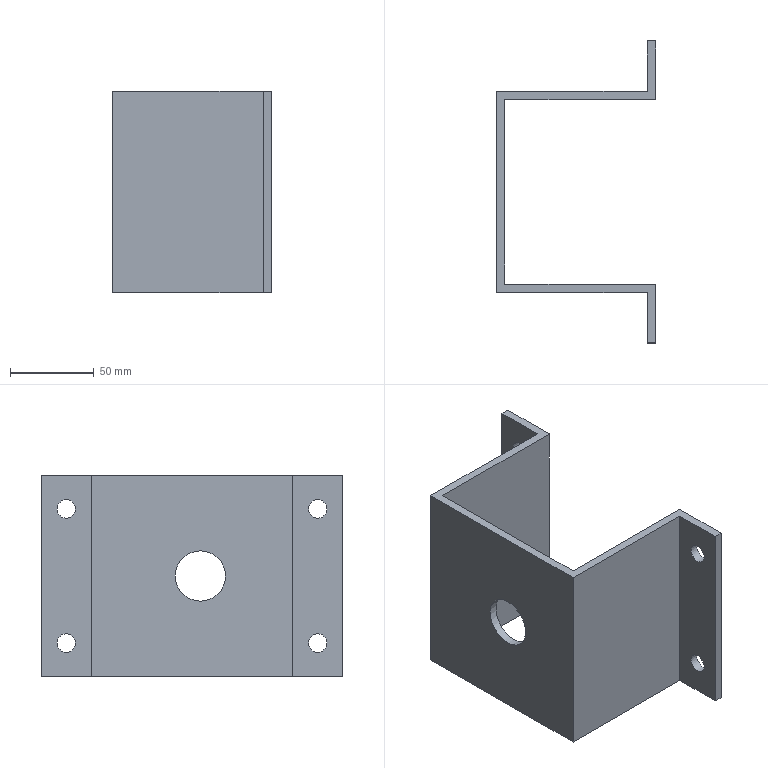Part | NX | features solid 2 | 1 solid | 19 faces | box 95 x 180 x 120 mm | volume 210565 mm3 | plane 14 | cylinder 5 | commonest cylinder face diameters 11 x4 30 x1
STEP:
#1=CARTESIAN_POINT('',(1255.,-598.,-435.));
#2=VERTEX_POINT('',#1);
#3=CARTESIAN_POINT('',(1255.,-598.,-315.));
#4=VERTEX_POINT('',#3);
#5=CARTESIAN_POINT('',(1255.,-598.,-435.));
#6=DIRECTION('',(0.,0.,1.));
#7=VECTOR('',#6,1000.);
#8=LINE('',#5,#7);
#9=EDGE_CURVE('',#2,#4,#8,.T.);
#10=ORIENTED_EDGE('',*,*,#9,.T.);
#11=CARTESIAN_POINT('',(1165.,-598.,-315.));
#12=VERTEX_POINT('',#11);
#13=CARTESIAN_POINT('',(1255.,-598.,-315.));
#14=DIRECTION('',(-1.,0.,0.));
#15=VECTOR('',#14,1000.);
#16=LINE('',#13,#15);
#17=EDGE_CURVE('',#4,#12,#16,.T.);
#18=ORIENTED_EDGE('',*,*,#17,.T.);
#19=CARTESIAN_POINT('',(1165.,-598.,-435.));
#20=VERTEX_POINT('',#19);
#21=CARTESIAN_POINT('',(1165.,-598.,-435.));
#22=DIRECTION('',(0.,0.,1.));
#23=VECTOR('',#22,1000.);
#24=LINE('',#21,#23);
#25=EDGE_CURVE('',#20,#12,#24,.T.);
#26=ORIENTED_EDGE('',*,*,#25,.F.);
#27=CARTESIAN_POINT('',(1255.,-598.,-435.));
#28=DIRECTION('',(-1.,0.,0.));
#29=VECTOR('',#28,1000.);
#30=LINE('',#27,#29);
#31=EDGE_CURVE('',#2,#20,#30,.T.);
#32=ORIENTED_EDGE('',*,*,#31,.F.);
#33=EDGE_LOOP('',(#10,#18,#26,#32));
#34=FACE_BOUND('',#33,.T.);
#35=CARTESIAN_POINT('',(1255.,-598.,-435.));
#36=DIRECTION('',(0.,1.,0.));
#37=DIRECTION('',(0.,0.,1.));
#38=AXIS2_PLACEMENT_3D('',#35,#36,#37);
#39=PLANE('',#38);
#40=ADVANCED_FACE('',(#34),#39,.F.);
#41=CARTESIAN_POINT('',(1165.,-478.,-435.));
#42=VERTEX_POINT('',#41);
#43=CARTESIAN_POINT('',(1165.,-598.,-435.));
#44=DIRECTION('',(0.,1.,0.));
#45=VECTOR('',#44,1000.);
#46=LINE('',#43,#45);
#47=EDGE_CURVE('',#20,#42,#46,.T.);
#48=ORIENTED_EDGE('',*,*,#47,.T.);
#49=CARTESIAN_POINT('',(1255.,-478.,-435.));
#50=VERTEX_POINT('',#49);
#51=CARTESIAN_POINT('',(1255.,-478.,-435.));
#52=DIRECTION('',(-1.,0.,0.));
#53=VECTOR('',#52,1000.);
#54=LINE('',#51,#53);
#55=EDGE_CURVE('',#50,#42,#54,.T.);
#56=ORIENTED_EDGE('',*,*,#55,.F.);
#57=CARTESIAN_POINT('',(1255.,-448.,-435.));
#58=VERTEX_POINT('',#57);
#59=CARTESIAN_POINT('',(1255.,-478.,-435.));
#60=DIRECTION('',(0.,-1.,0.));
#61=VECTOR('',#60,1000.);
#62=LINE('',#59,#61);
#63=EDGE_CURVE('',#50,#58,#62,.F.);
#64=ORIENTED_EDGE('',*,*,#63,.T.);
#65=CARTESIAN_POINT('',(1260.,-448.,-435.));
#66=VERTEX_POINT('',#65);
#67=CARTESIAN_POINT('',(1255.,-448.,-435.));
#68=DIRECTION('',(-1.,0.,0.));
#69=VECTOR('',#68,1000.);
#70=LINE('',#67,#69);
#71=EDGE_CURVE('',#66,#58,#70,.T.);
#72=ORIENTED_EDGE('',*,*,#71,.F.);
#73=CARTESIAN_POINT('',(1260.,-483.,-435.));
#74=VERTEX_POINT('',#73);
#75=CARTESIAN_POINT('',(1260.,-478.,-435.));
#76=DIRECTION('',(0.,-1.,0.));
#77=VECTOR('',#76,1000.);
#78=LINE('',#75,#77);
#79=EDGE_CURVE('',#66,#74,#78,.T.);
#80=ORIENTED_EDGE('',*,*,#79,.T.);
#81=CARTESIAN_POINT('',(1170.,-483.,-435.));
#82=VERTEX_POINT('',#81);
#83=CARTESIAN_POINT('',(1255.,-483.,-435.));
#84=DIRECTION('',(-1.,0.,0.));
#85=VECTOR('',#84,1000.);
#86=LINE('',#83,#85);
#87=EDGE_CURVE('',#74,#82,#86,.T.);
#88=ORIENTED_EDGE('',*,*,#87,.T.);
#89=CARTESIAN_POINT('',(1170.,-593.,-435.));
#90=VERTEX_POINT('',#89);
#91=CARTESIAN_POINT('',(1170.,-598.,-435.));
#92=DIRECTION('',(0.,1.,0.));
#93=VECTOR('',#92,1000.);
#94=LINE('',#91,#93);
#95=EDGE_CURVE('',#90,#82,#94,.T.);
#96=ORIENTED_EDGE('',*,*,#95,.F.);
#97=CARTESIAN_POINT('',(1260.,-593.,-435.));
#98=VERTEX_POINT('',#97);
#99=CARTESIAN_POINT('',(1255.,-593.,-435.));
#100=DIRECTION('',(-1.,0.,0.));
#101=VECTOR('',#100,1000.);
#102=LINE('',#99,#101);
#103=EDGE_CURVE('',#98,#90,#102,.T.);
#104=ORIENTED_EDGE('',*,*,#103,.F.);
#105=CARTESIAN_POINT('',(1260.,-628.,-435.));
#106=VERTEX_POINT('',#105);
#107=CARTESIAN_POINT('',(1260.,-598.,-435.));
#108=DIRECTION('',(0.,1.,0.));
#109=VECTOR('',#108,1000.);
#110=LINE('',#107,#109);
#111=EDGE_CURVE('',#106,#98,#110,.T.);
#112=ORIENTED_EDGE('',*,*,#111,.F.);
#113=CARTESIAN_POINT('',(1255.,-628.,-435.));
#114=VERTEX_POINT('',#113);
#115=CARTESIAN_POINT('',(1255.,-628.,-435.));
#116=DIRECTION('',(-1.,0.,0.));
#117=VECTOR('',#116,1000.);
#118=LINE('',#115,#117);
#119=EDGE_CURVE('',#106,#114,#118,.T.);
#120=ORIENTED_EDGE('',*,*,#119,.T.);
#121=CARTESIAN_POINT('',(1255.,-598.,-435.));
#122=DIRECTION('',(0.,1.,0.));
#123=VECTOR('',#122,1000.);
#124=LINE('',#121,#123);
#125=EDGE_CURVE('',#2,#114,#124,.F.);
#126=ORIENTED_EDGE('',*,*,#125,.F.);
#127=ORIENTED_EDGE('',*,*,#31,.T.);
#128=EDGE_LOOP('',(#48,#56,#64,#72,#80,#88,#96,#104,#112,#120,#126,#127));
#129=FACE_BOUND('',#128,.T.);
#130=CARTESIAN_POINT('',(1255.,-598.,-435.));
#131=DIRECTION('',(0.,0.,1.));
#132=DIRECTION('',(1.,0.,0.));
#133=AXIS2_PLACEMENT_3D('',#130,#131,#132);
#134=PLANE('',#133);
#135=ADVANCED_FACE('',(#129),#134,.F.);
#136=CARTESIAN_POINT('',(1260.,-613.,-420.5));
#137=VERTEX_POINT('',#136);
#138=CARTESIAN_POINT('',(1260.,-613.,-415.));
#139=DIRECTION('',(1.,0.,0.));
#140=DIRECTION('',(0.,0.,-1.));
#141=AXIS2_PLACEMENT_3D('',#138,#139,#140);
#142=CIRCLE('',#141,5.5);
#143=EDGE_CURVE('',#137,#137,#142,.T.);
#144=ORIENTED_EDGE('',*,*,#143,.F.);
#145=EDGE_LOOP('',(#144));
#146=FACE_BOUND('',#145,.T.);
#147=CARTESIAN_POINT('',(1260.,-613.,-340.5));
#148=VERTEX_POINT('',#147);
#149=CARTESIAN_POINT('',(1260.,-613.,-335.));
#150=DIRECTION('',(1.,0.,0.));
#151=DIRECTION('',(0.,0.,-1.));
#152=AXIS2_PLACEMENT_3D('',#149,#150,#151);
#153=CIRCLE('',#152,5.5);
#154=EDGE_CURVE('',#148,#148,#153,.T.);
#155=ORIENTED_EDGE('',*,*,#154,.F.);
#156=EDGE_LOOP('',(#155));
#157=FACE_BOUND('',#156,.T.);
#158=CARTESIAN_POINT('',(1260.,-593.,-315.));
#159=VERTEX_POINT('',#158);
#160=CARTESIAN_POINT('',(1260.,-593.,-435.));
#161=DIRECTION('',(0.,0.,1.));
#162=VECTOR('',#161,1000.);
#163=LINE('',#160,#162);
#164=EDGE_CURVE('',#98,#159,#163,.T.);
#165=ORIENTED_EDGE('',*,*,#164,.T.);
#166=CARTESIAN_POINT('',(1260.,-628.,-315.));
#167=VERTEX_POINT('',#166);
#168=CARTESIAN_POINT('',(1260.,-598.,-315.));
#169=DIRECTION('',(0.,1.,0.));
#170=VECTOR('',#169,1000.);
#171=LINE('',#168,#170);
#172=EDGE_CURVE('',#167,#159,#171,.T.);
#173=ORIENTED_EDGE('',*,*,#172,.F.);
#174=CARTESIAN_POINT('',(1260.,-628.,-435.));
#175=DIRECTION('',(0.,0.,1.));
#176=VECTOR('',#175,1000.);
#177=LINE('',#174,#176);
#178=EDGE_CURVE('',#106,#167,#177,.T.);
#179=ORIENTED_EDGE('',*,*,#178,.F.);
#180=ORIENTED_EDGE('',*,*,#111,.T.);
#181=EDGE_LOOP('',(#165,#173,#179,#180));
#182=FACE_BOUND('',#181,.T.);
#183=CARTESIAN_POINT('',(1260.,-598.,-435.));
#184=DIRECTION('',(1.,0.,0.));
#185=DIRECTION('',(0.,0.,-1.));
#186=AXIS2_PLACEMENT_3D('',#183,#184,#185);
#187=PLANE('',#186);
#188=ADVANCED_FACE('',(#146,#157,#182),#187,.T.);
#189=CARTESIAN_POINT('',(1170.,-593.,-315.));
#190=VERTEX_POINT('',#189);
#191=CARTESIAN_POINT('',(1170.,-483.,-315.));
#192=VERTEX_POINT('',#191);
#193=CARTESIAN_POINT('',(1170.,-598.,-315.));
#194=DIRECTION('',(0.,1.,0.));
#195=VECTOR('',#194,1000.);
#196=LINE('',#193,#195);
#197=EDGE_CURVE('',#190,#192,#196,.T.);
#198=ORIENTED_EDGE('',*,*,#197,.T.);
#199=CARTESIAN_POINT('',(1260.,-483.,-315.));
#200=VERTEX_POINT('',#199);
#201=CARTESIAN_POINT('',(1255.,-483.,-315.));
#202=DIRECTION('',(-1.,0.,0.));
#203=VECTOR('',#202,1000.);
#204=LINE('',#201,#203);
#205=EDGE_CURVE('',#200,#192,#204,.T.);
#206=ORIENTED_EDGE('',*,*,#205,.F.);
#207=CARTESIAN_POINT('',(1260.,-448.,-315.));
#208=VERTEX_POINT('',#207);
#209=CARTESIAN_POINT('',(1260.,-478.,-315.));
#210=DIRECTION('',(0.,-1.,0.));
#211=VECTOR('',#210,1000.);
#212=LINE('',#209,#211);
#213=EDGE_CURVE('',#208,#200,#212,.T.);
#214=ORIENTED_EDGE('',*,*,#213,.F.);
#215=CARTESIAN_POINT('',(1255.,-448.,-315.));
#216=VERTEX_POINT('',#215);
#217=CARTESIAN_POINT('',(1255.,-448.,-315.));
#218=DIRECTION('',(-1.,0.,0.));
#219=VECTOR('',#218,1000.);
#220=LINE('',#217,#219);
#221=EDGE_CURVE('',#208,#216,#220,.T.);
#222=ORIENTED_EDGE('',*,*,#221,.T.);
#223=CARTESIAN_POINT('',(1255.,-478.,-315.));
#224=VERTEX_POINT('',#223);
#225=CARTESIAN_POINT('',(1255.,-478.,-315.));
#226=DIRECTION('',(0.,-1.,0.));
#227=VECTOR('',#226,1000.);
#228=LINE('',#225,#227);
#229=EDGE_CURVE('',#224,#216,#228,.F.);
#230=ORIENTED_EDGE('',*,*,#229,.F.);
#231=CARTESIAN_POINT('',(1165.,-478.,-315.));
#232=VERTEX_POINT('',#231);
#233=CARTESIAN_POINT('',(1255.,-478.,-315.));
#234=DIRECTION('',(-1.,0.,0.));
#235=VECTOR('',#234,1000.);
#236=LINE('',#233,#235);
#237=EDGE_CURVE('',#224,#232,#236,.T.);
#238=ORIENTED_EDGE('',*,*,#237,.T.);
#239=CARTESIAN_POINT('',(1165.,-598.,-315.));
#240=DIRECTION('',(0.,1.,0.));
#241=VECTOR('',#240,1000.);
#242=LINE('',#239,#241);
#243=EDGE_CURVE('',#12,#232,#242,.T.);
#244=ORIENTED_EDGE('',*,*,#243,.F.);
#245=ORIENTED_EDGE('',*,*,#17,.F.);
#246=CARTESIAN_POINT('',(1255.,-628.,-315.));
#247=VERTEX_POINT('',#246);
#248=CARTESIAN_POINT('',(1255.,-598.,-315.));
#249=DIRECTION('',(0.,1.,0.));
#250=VECTOR('',#249,1000.);
#251=LINE('',#248,#250);
#252=EDGE_CURVE('',#4,#247,#251,.F.);
#253=ORIENTED_EDGE('',*,*,#252,.T.);
#254=CARTESIAN_POINT('',(1255.,-628.,-315.));
#255=DIRECTION('',(-1.,0.,0.));
#256=VECTOR('',#255,1000.);
#257=LINE('',#254,#256);
#258=EDGE_CURVE('',#167,#247,#257,.T.);
#259=ORIENTED_EDGE('',*,*,#258,.F.);
#260=ORIENTED_EDGE('',*,*,#172,.T.);
#261=CARTESIAN_POINT('',(1255.,-593.,-315.));
#262=DIRECTION('',(-1.,0.,0.));
#263=VECTOR('',#262,1000.);
#264=LINE('',#261,#263);
#265=EDGE_CURVE('',#159,#190,#264,.T.);
#266=ORIENTED_EDGE('',*,*,#265,.T.);
#267=EDGE_LOOP('',(#198,#206,#214,#222,#230,#238,#244,#245,#253,#259,#260,#266));
#268=FACE_BOUND('',#267,.T.);
#269=CARTESIAN_POINT('',(1255.,-598.,-315.));
#270=DIRECTION('',(0.,0.,1.));
#271=DIRECTION('',(1.,0.,0.));
#272=AXIS2_PLACEMENT_3D('',#269,#270,#271);
#273=PLANE('',#272);
#274=ADVANCED_FACE('',(#268),#273,.T.);
#275=CARTESIAN_POINT('',(1170.,-593.,-435.));
#276=DIRECTION('',(0.,0.,1.));
#277=VECTOR('',#276,1000.);
#278=LINE('',#275,#277);
#279=EDGE_CURVE('',#90,#190,#278,.T.);
#280=ORIENTED_EDGE('',*,*,#279,.T.);
#281=ORIENTED_EDGE('',*,*,#265,.F.);
#282=ORIENTED_EDGE('',*,*,#164,.F.);
#283=ORIENTED_EDGE('',*,*,#103,.T.);
#284=EDGE_LOOP('',(#280,#281,#282,#283));
#285=FACE_BOUND('',#284,.T.);
#286=CARTESIAN_POINT('',(1255.,-593.,-435.));
#287=DIRECTION('',(0.,1.,0.));
#288=DIRECTION('',(0.,0.,1.));
#289=AXIS2_PLACEMENT_3D('',#286,#287,#288);
#290=PLANE('',#289);
#291=ADVANCED_FACE('',(#285),#290,.T.);
#292=CARTESIAN_POINT('',(1255.,-613.,-420.5));
#293=VERTEX_POINT('',#292);
#294=CARTESIAN_POINT('',(1255.,-613.,-415.));
#295=DIRECTION('',(1.,0.,0.));
#296=DIRECTION('',(0.,0.,-1.));
#297=AXIS2_PLACEMENT_3D('',#294,#295,#296);
#298=CIRCLE('',#297,5.5);
#299=EDGE_CURVE('',#293,#293,#298,.T.);
#300=ORIENTED_EDGE('',*,*,#299,.T.);
#301=EDGE_LOOP('',(#300));
#302=FACE_BOUND('',#301,.T.);
#303=CARTESIAN_POINT('',(1255.,-613.,-340.5));
#304=VERTEX_POINT('',#303);
#305=CARTESIAN_POINT('',(1255.,-613.,-335.));
#306=DIRECTION('',(1.,0.,0.));
#307=DIRECTION('',(0.,0.,-1.));
#308=AXIS2_PLACEMENT_3D('',#305,#306,#307);
#309=CIRCLE('',#308,5.5);
#310=EDGE_CURVE('',#304,#304,#309,.T.);
#311=ORIENTED_EDGE('',*,*,#310,.T.);
#312=EDGE_LOOP('',(#311));
#313=FACE_BOUND('',#312,.T.);
#314=ORIENTED_EDGE('',*,*,#252,.F.);
#315=ORIENTED_EDGE('',*,*,#9,.F.);
#316=ORIENTED_EDGE('',*,*,#125,.T.);
#317=CARTESIAN_POINT('',(1255.,-628.,-435.));
#318=DIRECTION('',(0.,0.,1.));
#319=VECTOR('',#318,1000.);
#320=LINE('',#317,#319);
#321=EDGE_CURVE('',#114,#247,#320,.T.);
#322=ORIENTED_EDGE('',*,*,#321,.T.);
#323=EDGE_LOOP('',(#314,#315,#316,#322));
#324=FACE_BOUND('',#323,.T.);
#325=CARTESIAN_POINT('',(1255.,-598.,-435.));
#326=DIRECTION('',(1.,0.,0.));
#327=DIRECTION('',(0.,0.,1.));
#328=AXIS2_PLACEMENT_3D('',#325,#326,#327);
#329=PLANE('',#328);
#330=ADVANCED_FACE('',(#302,#313,#324),#329,.F.);
#331=ORIENTED_EDGE('',*,*,#321,.F.);
#332=ORIENTED_EDGE('',*,*,#119,.F.);
#333=ORIENTED_EDGE('',*,*,#178,.T.);
#334=ORIENTED_EDGE('',*,*,#258,.T.);
#335=EDGE_LOOP('',(#331,#332,#333,#334));
#336=FACE_BOUND('',#335,.T.);
#337=CARTESIAN_POINT('',(1255.,-628.,-435.));
#338=DIRECTION('',(0.,1.,0.));
#339=DIRECTION('',(0.,0.,1.));
#340=AXIS2_PLACEMENT_3D('',#337,#338,#339);
#341=PLANE('',#340);
#342=ADVANCED_FACE('',(#336),#341,.F.);
#343=CARTESIAN_POINT('',(1170.,-543.,-390.));
#344=VERTEX_POINT('',#343);
#345=CARTESIAN_POINT('',(1170.,-543.,-375.));
#346=DIRECTION('',(1.,0.,0.));
#347=DIRECTION('',(0.,0.,-1.));
#348=AXIS2_PLACEMENT_3D('',#345,#346,#347);
#349=CIRCLE('',#348,15.);
#350=EDGE_CURVE('',#344,#344,#349,.T.);
#351=ORIENTED_EDGE('',*,*,#350,.F.);
#352=EDGE_LOOP('',(#351));
#353=FACE_BOUND('',#352,.T.);
#354=ORIENTED_EDGE('',*,*,#95,.T.);
#355=CARTESIAN_POINT('',(1170.,-483.,-435.));
#356=DIRECTION('',(0.,0.,1.));
#357=VECTOR('',#356,1000.);
#358=LINE('',#355,#357);
#359=EDGE_CURVE('',#82,#192,#358,.T.);
#360=ORIENTED_EDGE('',*,*,#359,.T.);
#361=ORIENTED_EDGE('',*,*,#197,.F.);
#362=ORIENTED_EDGE('',*,*,#279,.F.);
#363=EDGE_LOOP('',(#354,#360,#361,#362));
#364=FACE_BOUND('',#363,.T.);
#365=CARTESIAN_POINT('',(1170.,-598.,-435.));
#366=DIRECTION('',(1.,0.,0.));
#367=DIRECTION('',(0.,0.,-1.));
#368=AXIS2_PLACEMENT_3D('',#365,#366,#367);
#369=PLANE('',#368);
#370=ADVANCED_FACE('',(#353,#364),#369,.T.);
#371=CARTESIAN_POINT('',(1165.,-543.,-390.));
#372=VERTEX_POINT('',#371);
#373=CARTESIAN_POINT('',(1165.,-543.,-375.));
#374=DIRECTION('',(1.,0.,0.));
#375=DIRECTION('',(0.,0.,-1.));
#376=AXIS2_PLACEMENT_3D('',#373,#374,#375);
#377=CIRCLE('',#376,15.);
#378=EDGE_CURVE('',#372,#372,#377,.T.);
#379=ORIENTED_EDGE('',*,*,#378,.T.);
#380=EDGE_LOOP('',(#379));
#381=FACE_BOUND('',#380,.T.);
#382=ORIENTED_EDGE('',*,*,#243,.T.);
#383=CARTESIAN_POINT('',(1165.,-478.,-435.));
#384=DIRECTION('',(0.,0.,1.));
#385=VECTOR('',#384,1000.);
#386=LINE('',#383,#385);
#387=EDGE_CURVE('',#42,#232,#386,.T.);
#388=ORIENTED_EDGE('',*,*,#387,.F.);
#389=ORIENTED_EDGE('',*,*,#47,.F.);
#390=ORIENTED_EDGE('',*,*,#25,.T.);
#391=EDGE_LOOP('',(#382,#388,#389,#390));
#392=FACE_BOUND('',#391,.T.);
#393=CARTESIAN_POINT('',(1165.,-598.,-435.));
#394=DIRECTION('',(1.,0.,0.));
#395=DIRECTION('',(0.,0.,-1.));
#396=AXIS2_PLACEMENT_3D('',#393,#394,#395);
#397=PLANE('',#396);
#398=ADVANCED_FACE('',(#381,#392),#397,.F.);
#399=CARTESIAN_POINT('',(1255.,-478.,-435.));
#400=DIRECTION('',(0.,0.,1.));
#401=VECTOR('',#400,1000.);
#402=LINE('',#399,#401);
#403=EDGE_CURVE('',#50,#224,#402,.T.);
#404=ORIENTED_EDGE('',*,*,#403,.F.);
#405=ORIENTED_EDGE('',*,*,#55,.T.);
#406=ORIENTED_EDGE('',*,*,#387,.T.);
#407=ORIENTED_EDGE('',*,*,#237,.F.);
#408=EDGE_LOOP('',(#404,#405,#406,#407));
#409=FACE_BOUND('',#408,.T.);
#410=CARTESIAN_POINT('',(1255.,-478.,-435.));
#411=DIRECTION('',(0.,-1.,0.));
#412=DIRECTION('',(0.,0.,1.));
#413=AXIS2_PLACEMENT_3D('',#410,#411,#412);
#414=PLANE('',#413);
#415=ADVANCED_FACE('',(#409),#414,.F.);
#416=CARTESIAN_POINT('',(1260.,-463.,-420.5));
#417=VERTEX_POINT('',#416);
#418=CARTESIAN_POINT('',(1260.,-463.,-415.));
#419=DIRECTION('',(1.,0.,0.));
#420=DIRECTION('',(0.,0.,-1.));
#421=AXIS2_PLACEMENT_3D('',#418,#419,#420);
#422=CIRCLE('',#421,5.5);
#423=EDGE_CURVE('',#417,#417,#422,.T.);
#424=ORIENTED_EDGE('',*,*,#423,.F.);
#425=EDGE_LOOP('',(#424));
#426=FACE_BOUND('',#425,.T.);
#427=CARTESIAN_POINT('',(1260.,-463.,-340.5));
#428=VERTEX_POINT('',#427);
#429=CARTESIAN_POINT('',(1260.,-463.,-335.));
#430=DIRECTION('',(1.,0.,0.));
#431=DIRECTION('',(0.,0.,-1.));
#432=AXIS2_PLACEMENT_3D('',#429,#430,#431);
#433=CIRCLE('',#432,5.5);
#434=EDGE_CURVE('',#428,#428,#433,.T.);
#435=ORIENTED_EDGE('',*,*,#434,.F.);
#436=EDGE_LOOP('',(#435));
#437=FACE_BOUND('',#436,.T.);
#438=CARTESIAN_POINT('',(1260.,-483.,-435.));
#439=DIRECTION('',(0.,0.,1.));
#440=VECTOR('',#439,1000.);
#441=LINE('',#438,#440);
#442=EDGE_CURVE('',#74,#200,#441,.T.);
#443=ORIENTED_EDGE('',*,*,#442,.F.);
#444=ORIENTED_EDGE('',*,*,#79,.F.);
#445=CARTESIAN_POINT('',(1260.,-448.,-435.));
#446=DIRECTION('',(0.,0.,1.));
#447=VECTOR('',#446,1000.);
#448=LINE('',#445,#447);
#449=EDGE_CURVE('',#66,#208,#448,.T.);
#450=ORIENTED_EDGE('',*,*,#449,.T.);
#451=ORIENTED_EDGE('',*,*,#213,.T.);
#452=EDGE_LOOP('',(#443,#444,#450,#451));
#453=FACE_BOUND('',#452,.T.);
#454=CARTESIAN_POINT('',(1260.,-478.,-435.));
#455=DIRECTION('',(1.,0.,0.));
#456=DIRECTION('',(0.,0.,-1.));
#457=AXIS2_PLACEMENT_3D('',#454,#455,#456);
#458=PLANE('',#457);
#459=ADVANCED_FACE('',(#426,#437,#453),#458,.T.);
#460=ORIENTED_EDGE('',*,*,#359,.F.);
#461=ORIENTED_EDGE('',*,*,#87,.F.);
#462=ORIENTED_EDGE('',*,*,#442,.T.);
#463=ORIENTED_EDGE('',*,*,#205,.T.);
#464=EDGE_LOOP('',(#460,#461,#462,#463));
#465=FACE_BOUND('',#464,.T.);
#466=CARTESIAN_POINT('',(1255.,-483.,-435.));
#467=DIRECTION('',(0.,-1.,0.));
#468=DIRECTION('',(0.,0.,1.));
#469=AXIS2_PLACEMENT_3D('',#466,#467,#468);
#470=PLANE('',#469);
#471=ADVANCED_FACE('',(#465),#470,.T.);
#472=CARTESIAN_POINT('',(1255.,-463.,-420.5));
#473=VERTEX_POINT('',#472);
#474=CARTESIAN_POINT('',(1255.,-463.,-415.));
#475=DIRECTION('',(1.,0.,0.));
#476=DIRECTION('',(0.,0.,-1.));
#477=AXIS2_PLACEMENT_3D('',#474,#475,#476);
#478=CIRCLE('',#477,5.5);
#479=EDGE_CURVE('',#473,#473,#478,.T.);
#480=ORIENTED_EDGE('',*,*,#479,.T.);
#481=EDGE_LOOP('',(#480));
#482=FACE_BOUND('',#481,.T.);
#483=CARTESIAN_POINT('',(1255.,-463.,-340.5));
#484=VERTEX_POINT('',#483);
#485=CARTESIAN_POINT('',(1255.,-463.,-335.));
#486=DIRECTION('',(1.,0.,0.));
#487=DIRECTION('',(0.,0.,-1.));
#488=AXIS2_PLACEMENT_3D('',#485,#486,#487);
#489=CIRCLE('',#488,5.5);
#490=EDGE_CURVE('',#484,#484,#489,.T.);
#491=ORIENTED_EDGE('',*,*,#490,.T.);
#492=EDGE_LOOP('',(#491));
#493=FACE_BOUND('',#492,.T.);
#494=ORIENTED_EDGE('',*,*,#229,.T.);
#495=CARTESIAN_POINT('',(1255.,-448.,-435.));
#496=DIRECTION('',(0.,0.,1.));
#497=VECTOR('',#496,1000.);
#498=LINE('',#495,#497);
#499=EDGE_CURVE('',#58,#216,#498,.T.);
#500=ORIENTED_EDGE('',*,*,#499,.F.);
#501=ORIENTED_EDGE('',*,*,#63,.F.);
#502=ORIENTED_EDGE('',*,*,#403,.T.);
#503=EDGE_LOOP('',(#494,#500,#501,#502));
#504=FACE_BOUND('',#503,.T.);
#505=CARTESIAN_POINT('',(1255.,-478.,-435.));
#506=DIRECTION('',(1.,0.,0.));
#507=DIRECTION('',(0.,0.,1.));
#508=AXIS2_PLACEMENT_3D('',#505,#506,#507);
#509=PLANE('',#508);
#510=ADVANCED_FACE('',(#482,#493,#504),#509,.F.);
#511=ORIENTED_EDGE('',*,*,#499,.T.);
#512=ORIENTED_EDGE('',*,*,#221,.F.);
#513=ORIENTED_EDGE('',*,*,#449,.F.);
#514=ORIENTED_EDGE('',*,*,#71,.T.);
#515=EDGE_LOOP('',(#511,#512,#513,#514));
#516=FACE_BOUND('',#515,.T.);
#517=CARTESIAN_POINT('',(1255.,-448.,-435.));
#518=DIRECTION('',(0.,-1.,0.));
#519=DIRECTION('',(0.,0.,1.));
#520=AXIS2_PLACEMENT_3D('',#517,#518,#519);
#521=PLANE('',#520);
#522=ADVANCED_FACE('',(#516),#521,.F.);
#523=ORIENTED_EDGE('',*,*,#350,.T.);
#524=EDGE_LOOP('',(#523));
#525=FACE_BOUND('',#524,.T.);
#526=ORIENTED_EDGE('',*,*,#378,.F.);
#527=EDGE_LOOP('',(#526));
#528=FACE_BOUND('',#527,.T.);
#529=CARTESIAN_POINT('',(1165.,-543.,-375.));
#530=DIRECTION('',(1.,0.,0.));
#531=DIRECTION('',(0.,0.,-1.));
#532=AXIS2_PLACEMENT_3D('',#529,#530,#531);
#533=CYLINDRICAL_SURFACE('',#532,15.);
#534=ADVANCED_FACE('',(#525,#528),#533,.F.);
#535=ORIENTED_EDGE('',*,*,#154,.T.);
#536=EDGE_LOOP('',(#535));
#537=FACE_BOUND('',#536,.T.);
#538=ORIENTED_EDGE('',*,*,#310,.F.);
#539=EDGE_LOOP('',(#538));
#540=FACE_BOUND('',#539,.T.);
#541=CARTESIAN_POINT('',(1210.,-613.,-335.));
#542=DIRECTION('',(1.,0.,0.));
#543=DIRECTION('',(0.,0.,-1.));
#544=AXIS2_PLACEMENT_3D('',#541,#542,#543);
#545=CYLINDRICAL_SURFACE('',#544,5.5);
#546=ADVANCED_FACE('',(#537,#540),#545,.F.);
#547=ORIENTED_EDGE('',*,*,#143,.T.);
#548=EDGE_LOOP('',(#547));
#549=FACE_BOUND('',#548,.T.);
#550=ORIENTED_EDGE('',*,*,#299,.F.);
#551=EDGE_LOOP('',(#550));
#552=FACE_BOUND('',#551,.T.);
#553=CARTESIAN_POINT('',(1210.,-613.,-415.));
#554=DIRECTION('',(1.,0.,0.));
#555=DIRECTION('',(0.,0.,-1.));
#556=AXIS2_PLACEMENT_3D('',#553,#554,#555);
#557=CYLINDRICAL_SURFACE('',#556,5.5);
#558=ADVANCED_FACE('',(#549,#552),#557,.F.);
#559=ORIENTED_EDGE('',*,*,#434,.T.);
#560=EDGE_LOOP('',(#559));
#561=FACE_BOUND('',#560,.T.);
#562=ORIENTED_EDGE('',*,*,#490,.F.);
#563=EDGE_LOOP('',(#562));
#564=FACE_BOUND('',#563,.T.);
#565=CARTESIAN_POINT('',(1210.,-463.,-335.));
#566=DIRECTION('',(1.,0.,0.));
#567=DIRECTION('',(0.,0.,-1.));
#568=AXIS2_PLACEMENT_3D('',#565,#566,#567);
#569=CYLINDRICAL_SURFACE('',#568,5.5);
#570=ADVANCED_FACE('',(#561,#564),#569,.F.);
#571=ORIENTED_EDGE('',*,*,#423,.T.);
#572=EDGE_LOOP('',(#571));
#573=FACE_BOUND('',#572,.T.);
#574=ORIENTED_EDGE('',*,*,#479,.F.);
#575=EDGE_LOOP('',(#574));
#576=FACE_BOUND('',#575,.T.);
#577=CARTESIAN_POINT('',(1210.,-463.,-415.));
#578=DIRECTION('',(1.,0.,0.));
#579=DIRECTION('',(0.,0.,-1.));
#580=AXIS2_PLACEMENT_3D('',#577,#578,#579);
#581=CYLINDRICAL_SURFACE('',#580,5.5);
#582=ADVANCED_FACE('',(#573,#576),#581,.F.);
#583=CLOSED_SHELL('',(#40,#135,#188,#274,#291,#330,#342,#370,#398,#415,#459,#471,#510,#522,#534,#546,#558,#570,#582));
#584=MANIFOLD_SOLID_BREP('',#583);
#585=(LENGTH_UNIT()NAMED_UNIT(*)SI_UNIT(.MILLI.,.METRE.));
#586=UNCERTAINTY_MEASURE_WITH_UNIT(LENGTH_MEASURE(0.00001),#585,'','');
#587=(NAMED_UNIT(*)PLANE_ANGLE_UNIT()SI_UNIT($,.RADIAN.));
#588=(NAMED_UNIT(*)SI_UNIT($,.STERADIAN.)SOLID_ANGLE_UNIT());
#589=(GEOMETRIC_REPRESENTATION_CONTEXT(3)GLOBAL_UNCERTAINTY_ASSIGNED_CONTEXT((#586))GLOBAL_UNIT_ASSIGNED_CONTEXT((#585,#587,#588))REPRESENTATION_CONTEXT('',''));
#590=ADVANCED_BREP_SHAPE_REPRESENTATION('',(#584),#589);